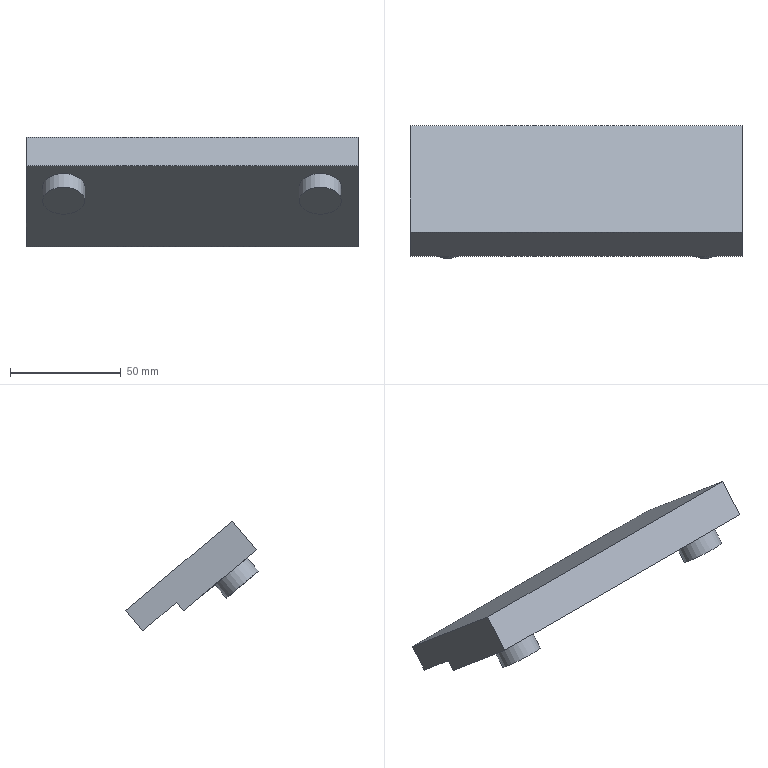Part | NX | features solid 2 | 1 solid | 12 faces | box 150 x 60.076 x 49.639 mm | volume 149580 mm3 | plane 10 | cylinder 2 | commonest cylinder face diameters 19 x2
STEP:
#1=CARTESIAN_POINT('',(65.,-309.05,-107.902));
#2=VERTEX_POINT('',#1);
#3=CARTESIAN_POINT('',(65.,-316.722,-117.046));
#4=VERTEX_POINT('',#3);
#5=CARTESIAN_POINT('',(65.,-307.08,-105.555));
#6=DIRECTION('',(0.,-0.6428,-0.766));
#7=VECTOR('',#6,1000.);
#8=LINE('',#5,#7);
#9=EDGE_CURVE('',#2,#4,#8,.T.);
#10=ORIENTED_EDGE('',*,*,#9,.T.);
#11=CARTESIAN_POINT('',(65.,-332.043,-104.19));
#12=VERTEX_POINT('',#11);
#13=CARTESIAN_POINT('',(65.,-316.722,-117.046));
#14=DIRECTION('',(0.,-0.766,0.6428));
#15=VECTOR('',#14,1000.);
#16=LINE('',#13,#15);
#17=EDGE_CURVE('',#4,#12,#16,.T.);
#18=ORIENTED_EDGE('',*,*,#17,.T.);
#19=CARTESIAN_POINT('',(65.,-335.257,-108.02));
#20=VERTEX_POINT('',#19);
#21=CARTESIAN_POINT('',(65.,-332.043,-104.19));
#22=DIRECTION('',(0.,0.6428,0.766));
#23=VECTOR('',#22,1000.);
#24=LINE('',#21,#23);
#25=EDGE_CURVE('',#12,#20,#24,.F.);
#26=ORIENTED_EDGE('',*,*,#25,.T.);
#27=CARTESIAN_POINT('',(65.,-368.197,-80.38));
#28=VERTEX_POINT('',#27);
#29=CARTESIAN_POINT('',(65.,-318.404,-122.161));
#30=DIRECTION('',(0.,-0.766,0.6428));
#31=VECTOR('',#30,1000.);
#32=LINE('',#29,#31);
#33=EDGE_CURVE('',#20,#28,#32,.T.);
#34=ORIENTED_EDGE('',*,*,#33,.T.);
#35=CARTESIAN_POINT('',(65.,-357.311,-67.407));
#36=VERTEX_POINT('',#35);
#37=CARTESIAN_POINT('',(65.,-355.341,-65.059));
#38=DIRECTION('',(0.,-0.6428,-0.766));
#39=VECTOR('',#38,1000.);
#40=LINE('',#37,#39);
#41=EDGE_CURVE('',#36,#28,#40,.T.);
#42=ORIENTED_EDGE('',*,*,#41,.F.);
#43=CARTESIAN_POINT('',(65.,-307.518,-109.188));
#44=DIRECTION('',(0.,0.766,-0.6428));
#45=VECTOR('',#44,1000.);
#46=LINE('',#43,#45);
#47=EDGE_CURVE('',#2,#36,#46,.F.);
#48=ORIENTED_EDGE('',*,*,#47,.F.);
#49=EDGE_LOOP('',(#10,#18,#26,#34,#42,#48));
#50=FACE_BOUND('',#49,.T.);
#51=CARTESIAN_POINT('',(65.,-305.548,-106.84));
#52=DIRECTION('',(1.,0.,0.));
#53=DIRECTION('',(0.,0.,-1.));
#54=AXIS2_PLACEMENT_3D('',#51,#52,#53);
#55=PLANE('',#54);
#56=ADVANCED_FACE('',(#50),#55,.F.);
#57=CARTESIAN_POINT('',(215.,-309.05,-107.902));
#58=VERTEX_POINT('',#57);
#59=CARTESIAN_POINT('',(215.,-316.722,-117.046));
#60=VERTEX_POINT('',#59);
#61=CARTESIAN_POINT('',(215.,-307.08,-105.555));
#62=DIRECTION('',(0.,-0.6428,-0.766));
#63=VECTOR('',#62,1000.);
#64=LINE('',#61,#63);
#65=EDGE_CURVE('',#58,#60,#64,.T.);
#66=ORIENTED_EDGE('',*,*,#65,.T.);
#67=CARTESIAN_POINT('',(215.,-316.722,-117.046));
#68=DIRECTION('',(-1.,0.,0.));
#69=VECTOR('',#68,1000.);
#70=LINE('',#67,#69);
#71=EDGE_CURVE('',#60,#4,#70,.T.);
#72=ORIENTED_EDGE('',*,*,#71,.T.);
#73=ORIENTED_EDGE('',*,*,#9,.F.);
#74=CARTESIAN_POINT('',(215.,-309.05,-107.902));
#75=DIRECTION('',(1.,0.,0.));
#76=VECTOR('',#75,1000.);
#77=LINE('',#74,#76);
#78=EDGE_CURVE('',#58,#2,#77,.F.);
#79=ORIENTED_EDGE('',*,*,#78,.F.);
#80=EDGE_LOOP('',(#66,#72,#73,#79));
#81=FACE_BOUND('',#80,.T.);
#82=CARTESIAN_POINT('',(215.,-307.08,-105.555));
#83=DIRECTION('',(0.,-0.766,0.6428));
#84=DIRECTION('',(0.,0.6428,0.766));
#85=AXIS2_PLACEMENT_3D('',#82,#83,#84);
#86=PLANE('',#85);
#87=ADVANCED_FACE('',(#81),#86,.F.);
#88=CARTESIAN_POINT('',(215.,-332.043,-104.19));
#89=VERTEX_POINT('',#88);
#90=CARTESIAN_POINT('',(215.,-316.722,-117.046));
#91=DIRECTION('',(0.,-0.766,0.6428));
#92=VECTOR('',#91,1000.);
#93=LINE('',#90,#92);
#94=EDGE_CURVE('',#60,#89,#93,.T.);
#95=ORIENTED_EDGE('',*,*,#94,.F.);
#96=ORIENTED_EDGE('',*,*,#65,.F.);
#97=CARTESIAN_POINT('',(215.,-357.311,-67.407));
#98=VERTEX_POINT('',#97);
#99=CARTESIAN_POINT('',(215.,-307.518,-109.188));
#100=DIRECTION('',(0.,0.766,-0.6428));
#101=VECTOR('',#100,1000.);
#102=LINE('',#99,#101);
#103=EDGE_CURVE('',#58,#98,#102,.F.);
#104=ORIENTED_EDGE('',*,*,#103,.T.);
#105=CARTESIAN_POINT('',(215.,-368.197,-80.38));
#106=VERTEX_POINT('',#105);
#107=CARTESIAN_POINT('',(215.,-355.341,-65.059));
#108=DIRECTION('',(0.,-0.6428,-0.766));
#109=VECTOR('',#108,1000.);
#110=LINE('',#107,#109);
#111=EDGE_CURVE('',#98,#106,#110,.T.);
#112=ORIENTED_EDGE('',*,*,#111,.T.);
#113=CARTESIAN_POINT('',(215.,-335.257,-108.02));
#114=VERTEX_POINT('',#113);
#115=CARTESIAN_POINT('',(215.,-318.404,-122.161));
#116=DIRECTION('',(0.,-0.766,0.6428));
#117=VECTOR('',#116,1000.);
#118=LINE('',#115,#117);
#119=EDGE_CURVE('',#114,#106,#118,.T.);
#120=ORIENTED_EDGE('',*,*,#119,.F.);
#121=CARTESIAN_POINT('',(215.,-332.043,-104.19));
#122=DIRECTION('',(0.,0.6428,0.766));
#123=VECTOR('',#122,1000.);
#124=LINE('',#121,#123);
#125=EDGE_CURVE('',#89,#114,#124,.F.);
#126=ORIENTED_EDGE('',*,*,#125,.F.);
#127=EDGE_LOOP('',(#95,#96,#104,#112,#120,#126));
#128=FACE_BOUND('',#127,.T.);
#129=CARTESIAN_POINT('',(215.,-305.548,-106.84));
#130=DIRECTION('',(1.,0.,0.));
#131=DIRECTION('',(0.,0.,-1.));
#132=AXIS2_PLACEMENT_3D('',#129,#130,#131);
#133=PLANE('',#132);
#134=ADVANCED_FACE('',(#128),#133,.T.);
#135=CARTESIAN_POINT('',(215.,-368.197,-80.38));
#136=DIRECTION('',(-1.,0.,0.));
#137=VECTOR('',#136,1000.);
#138=LINE('',#135,#137);
#139=EDGE_CURVE('',#106,#28,#138,.T.);
#140=ORIENTED_EDGE('',*,*,#139,.F.);
#141=ORIENTED_EDGE('',*,*,#111,.F.);
#142=CARTESIAN_POINT('',(215.,-357.311,-67.407));
#143=DIRECTION('',(1.,0.,0.));
#144=VECTOR('',#143,1000.);
#145=LINE('',#142,#144);
#146=EDGE_CURVE('',#98,#36,#145,.F.);
#147=ORIENTED_EDGE('',*,*,#146,.T.);
#148=ORIENTED_EDGE('',*,*,#41,.T.);
#149=EDGE_LOOP('',(#140,#141,#147,#148));
#150=FACE_BOUND('',#149,.T.);
#151=CARTESIAN_POINT('',(215.,-355.341,-65.059));
#152=DIRECTION('',(0.,-0.766,0.6428));
#153=DIRECTION('',(0.,0.6428,0.766));
#154=AXIS2_PLACEMENT_3D('',#151,#152,#153);
#155=PLANE('',#154);
#156=ADVANCED_FACE('',(#150),#155,.T.);
#157=ORIENTED_EDGE('',*,*,#47,.T.);
#158=ORIENTED_EDGE('',*,*,#146,.F.);
#159=ORIENTED_EDGE('',*,*,#103,.F.);
#160=ORIENTED_EDGE('',*,*,#78,.T.);
#161=EDGE_LOOP('',(#157,#158,#159,#160));
#162=FACE_BOUND('',#161,.T.);
#163=CARTESIAN_POINT('',(215.,-305.548,-110.84));
#164=DIRECTION('',(0.,-0.6428,-0.766));
#165=DIRECTION('',(0.,-0.766,0.6428));
#166=AXIS2_PLACEMENT_3D('',#163,#164,#165);
#167=PLANE('',#166);
#168=ADVANCED_FACE('',(#162),#167,.F.);
#169=CARTESIAN_POINT('',(215.,-335.257,-108.02));
#170=DIRECTION('',(-1.,0.,0.));
#171=VECTOR('',#170,1000.);
#172=LINE('',#169,#171);
#173=EDGE_CURVE('',#114,#20,#172,.T.);
#174=ORIENTED_EDGE('',*,*,#173,.F.);
#175=ORIENTED_EDGE('',*,*,#119,.T.);
#176=ORIENTED_EDGE('',*,*,#139,.T.);
#177=ORIENTED_EDGE('',*,*,#33,.F.);
#178=EDGE_LOOP('',(#174,#175,#176,#177));
#179=FACE_BOUND('',#178,.T.);
#180=CARTESIAN_POINT('',(198.,-363.983,-83.915));
#181=VERTEX_POINT('',#180);
#182=CARTESIAN_POINT('',(198.,-356.706,-90.022));
#183=DIRECTION('',(0.,-0.6428,-0.766));
#184=DIRECTION('',(0.,-0.766,0.6428));
#185=AXIS2_PLACEMENT_3D('',#182,#183,#184);
#186=CIRCLE('',#185,9.5);
#187=EDGE_CURVE('',#181,#181,#186,.T.);
#188=ORIENTED_EDGE('',*,*,#187,.F.);
#189=EDGE_LOOP('',(#188));
#190=FACE_BOUND('',#189,.T.);
#191=CARTESIAN_POINT('',(82.,-363.983,-83.915));
#192=VERTEX_POINT('',#191);
#193=CARTESIAN_POINT('',(82.,-356.706,-90.022));
#194=DIRECTION('',(0.,-0.6428,-0.766));
#195=DIRECTION('',(0.,-0.766,0.6428));
#196=AXIS2_PLACEMENT_3D('',#193,#194,#195);
#197=CIRCLE('',#196,9.5);
#198=EDGE_CURVE('',#192,#192,#197,.T.);
#199=ORIENTED_EDGE('',*,*,#198,.F.);
#200=EDGE_LOOP('',(#199));
#201=FACE_BOUND('',#200,.T.);
#202=CARTESIAN_POINT('',(215.,-318.404,-122.161));
#203=DIRECTION('',(0.,-0.6428,-0.766));
#204=DIRECTION('',(0.,-0.766,0.6428));
#205=AXIS2_PLACEMENT_3D('',#202,#203,#204);
#206=PLANE('',#205);
#207=ADVANCED_FACE('',(#179,#190,#201),#206,.T.);
#208=CARTESIAN_POINT('',(82.,-369.126,-90.044));
#209=VERTEX_POINT('',#208);
#210=CARTESIAN_POINT('',(82.,-361.848,-96.15));
#211=DIRECTION('',(0.,-0.6428,-0.766));
#212=DIRECTION('',(0.,-0.766,0.6428));
#213=AXIS2_PLACEMENT_3D('',#210,#211,#212);
#214=CIRCLE('',#213,9.5);
#215=EDGE_CURVE('',#209,#209,#214,.T.);
#216=ORIENTED_EDGE('',*,*,#215,.T.);
#217=EDGE_LOOP('',(#216));
#218=FACE_BOUND('',#217,.T.);
#219=CARTESIAN_POINT('',(82.,-361.848,-96.15));
#220=DIRECTION('',(0.,-0.6428,-0.766));
#221=DIRECTION('',(0.,-0.766,0.6428));
#222=AXIS2_PLACEMENT_3D('',#219,#220,#221);
#223=PLANE('',#222);
#224=ADVANCED_FACE('',(#218),#223,.T.);
#225=ORIENTED_EDGE('',*,*,#215,.F.);
#226=EDGE_LOOP('',(#225));
#227=FACE_BOUND('',#226,.T.);
#228=ORIENTED_EDGE('',*,*,#198,.T.);
#229=EDGE_LOOP('',(#228));
#230=FACE_BOUND('',#229,.T.);
#231=CARTESIAN_POINT('',(82.,-356.706,-90.022));
#232=DIRECTION('',(0.,-0.6428,-0.766));
#233=DIRECTION('',(0.,-0.766,0.6428));
#234=AXIS2_PLACEMENT_3D('',#231,#232,#233);
#235=CYLINDRICAL_SURFACE('',#234,9.5);
#236=ADVANCED_FACE('',(#227,#230),#235,.T.);
#237=CARTESIAN_POINT('',(198.,-369.126,-90.044));
#238=VERTEX_POINT('',#237);
#239=CARTESIAN_POINT('',(198.,-361.848,-96.15));
#240=DIRECTION('',(0.,-0.6428,-0.766));
#241=DIRECTION('',(0.,-0.766,0.6428));
#242=AXIS2_PLACEMENT_3D('',#239,#240,#241);
#243=CIRCLE('',#242,9.5);
#244=EDGE_CURVE('',#238,#238,#243,.T.);
#245=ORIENTED_EDGE('',*,*,#244,.T.);
#246=EDGE_LOOP('',(#245));
#247=FACE_BOUND('',#246,.T.);
#248=CARTESIAN_POINT('',(198.,-361.848,-96.15));
#249=DIRECTION('',(0.,-0.6428,-0.766));
#250=DIRECTION('',(0.,-0.766,0.6428));
#251=AXIS2_PLACEMENT_3D('',#248,#249,#250);
#252=PLANE('',#251);
#253=ADVANCED_FACE('',(#247),#252,.T.);
#254=ORIENTED_EDGE('',*,*,#244,.F.);
#255=EDGE_LOOP('',(#254));
#256=FACE_BOUND('',#255,.T.);
#257=ORIENTED_EDGE('',*,*,#187,.T.);
#258=EDGE_LOOP('',(#257));
#259=FACE_BOUND('',#258,.T.);
#260=CARTESIAN_POINT('',(198.,-356.706,-90.022));
#261=DIRECTION('',(0.,-0.6428,-0.766));
#262=DIRECTION('',(0.,-0.766,0.6428));
#263=AXIS2_PLACEMENT_3D('',#260,#261,#262);
#264=CYLINDRICAL_SURFACE('',#263,9.5);
#265=ADVANCED_FACE('',(#256,#259),#264,.T.);
#266=ORIENTED_EDGE('',*,*,#94,.T.);
#267=CARTESIAN_POINT('',(215.,-332.043,-104.19));
#268=DIRECTION('',(-1.,0.,0.));
#269=VECTOR('',#268,1000.);
#270=LINE('',#267,#269);
#271=EDGE_CURVE('',#89,#12,#270,.T.);
#272=ORIENTED_EDGE('',*,*,#271,.T.);
#273=ORIENTED_EDGE('',*,*,#17,.F.);
#274=ORIENTED_EDGE('',*,*,#71,.F.);
#275=EDGE_LOOP('',(#266,#272,#273,#274));
#276=FACE_BOUND('',#275,.T.);
#277=CARTESIAN_POINT('',(215.,-316.722,-117.046));
#278=DIRECTION('',(0.,0.6428,0.766));
#279=DIRECTION('',(-1.,0.,0.));
#280=AXIS2_PLACEMENT_3D('',#277,#278,#279);
#281=PLANE('',#280);
#282=ADVANCED_FACE('',(#276),#281,.F.);
#283=ORIENTED_EDGE('',*,*,#173,.T.);
#284=ORIENTED_EDGE('',*,*,#25,.F.);
#285=ORIENTED_EDGE('',*,*,#271,.F.);
#286=ORIENTED_EDGE('',*,*,#125,.T.);
#287=EDGE_LOOP('',(#283,#284,#285,#286));
#288=FACE_BOUND('',#287,.T.);
#289=CARTESIAN_POINT('',(215.,-332.043,-104.19));
#290=DIRECTION('',(0.,-0.766,0.6428));
#291=DIRECTION('',(0.,0.6428,0.766));
#292=AXIS2_PLACEMENT_3D('',#289,#290,#291);
#293=PLANE('',#292);
#294=ADVANCED_FACE('',(#288),#293,.F.);
#295=CLOSED_SHELL('',(#56,#87,#134,#156,#168,#207,#224,#236,#253,#265,#282,#294));
#296=MANIFOLD_SOLID_BREP('',#295);
#297=(LENGTH_UNIT()NAMED_UNIT(*)SI_UNIT(.MILLI.,.METRE.));
#298=UNCERTAINTY_MEASURE_WITH_UNIT(LENGTH_MEASURE(0.00001),#297,'','');
#299=(NAMED_UNIT(*)PLANE_ANGLE_UNIT()SI_UNIT($,.RADIAN.));
#300=(NAMED_UNIT(*)SI_UNIT($,.STERADIAN.)SOLID_ANGLE_UNIT());
#301=(GEOMETRIC_REPRESENTATION_CONTEXT(3)GLOBAL_UNCERTAINTY_ASSIGNED_CONTEXT((#298))GLOBAL_UNIT_ASSIGNED_CONTEXT((#297,#299,#300))REPRESENTATION_CONTEXT('',''));
#302=ADVANCED_BREP_SHAPE_REPRESENTATION('',(#296),#301);